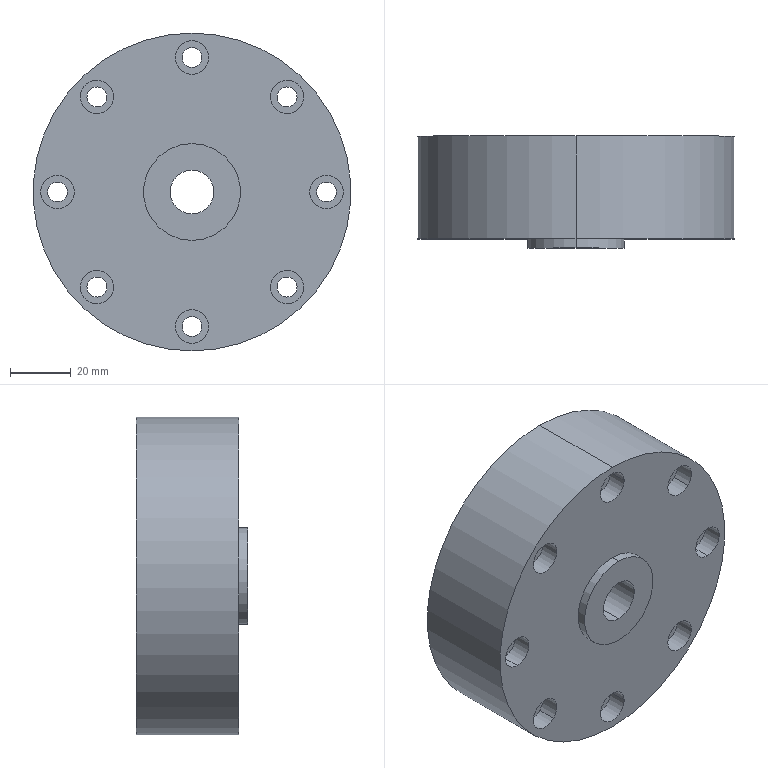Part | STEP file | NS-TH3B-3t | 1 solid | 49 faces | box 105 x 37 x 105 mm | volume 278290 mm3 | cylinder 38 | plane 11 | commonest cylinder face diameters 6.6 x16 11 x16 14.5 x2 32 x2 105 x2